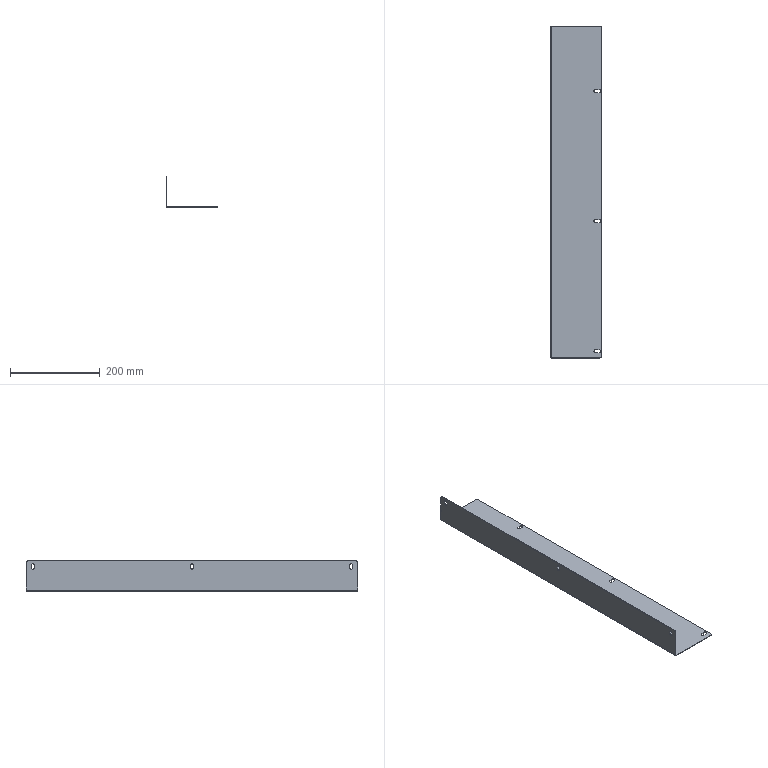Part | SolidWorks | features BaseBody 1 | 1 solid | 48 faces | box 115 x 740 x 67.2 mm | volume 159488 mm3 | cylinder 24 | plane 24 | commonest cylinder face diameters 7 x18 10 x4 2 x1 4.4 x1
STEP:
#1=CARTESIAN_POINT('',(55.,-355.,-1.2));
#2=VERTEX_POINT('',#1);
#3=CARTESIAN_POINT('',(51.5,-351.5,-1.2));
#4=VERTEX_POINT('',#3);
#5=CARTESIAN_POINT('',(51.5,-355.,-1.2));
#6=DIRECTION('',(0.,0.,1.));
#7=DIRECTION('',(1.,0.,0.));
#8=AXIS2_PLACEMENT_3D('',#5,#6,#7);
#9=CIRCLE('',#8,3.5);
#10=EDGE_CURVE('',#2,#4,#9,.T.);
#11=ORIENTED_EDGE('',*,*,#10,.F.);
#12=CARTESIAN_POINT('',(55.,-355.,0.));
#13=VERTEX_POINT('',#12);
#14=CARTESIAN_POINT('',(55.,-355.,-1.2));
#15=DIRECTION('',(0.,0.,1.));
#16=VECTOR('',#15,1000.);
#17=LINE('',#14,#16);
#18=EDGE_CURVE('',#2,#13,#17,.T.);
#19=ORIENTED_EDGE('',*,*,#18,.T.);
#20=CARTESIAN_POINT('',(51.5,-351.5,0.));
#21=VERTEX_POINT('',#20);
#22=CARTESIAN_POINT('',(51.5,-355.,0.));
#23=DIRECTION('',(0.,0.,1.));
#24=DIRECTION('',(1.,0.,0.));
#25=AXIS2_PLACEMENT_3D('',#22,#23,#24);
#26=CIRCLE('',#25,3.5);
#27=EDGE_CURVE('',#13,#21,#26,.T.);
#28=ORIENTED_EDGE('',*,*,#27,.T.);
#29=CARTESIAN_POINT('',(51.5,-351.5,-1.2));
#30=DIRECTION('',(0.,0.,1.));
#31=VECTOR('',#30,1000.);
#32=LINE('',#29,#31);
#33=EDGE_CURVE('',#4,#21,#32,.T.);
#34=ORIENTED_EDGE('',*,*,#33,.F.);
#35=EDGE_LOOP('',(#11,#19,#28,#34));
#36=FACE_OUTER_BOUND('',#35,.T.);
#37=CARTESIAN_POINT('',(51.5,-355.,-1.2));
#38=DIRECTION('',(0.,0.,1.));
#39=DIRECTION('',(1.,0.,0.));
#40=AXIS2_PLACEMENT_3D('',#37,#38,#39);
#41=CYLINDRICAL_SURFACE('',#40,3.5);
#42=ADVANCED_FACE('',(#36),#41,.F.);
#43=CARTESIAN_POINT('',(55.,-65.,-1.2));
#44=VERTEX_POINT('',#43);
#45=CARTESIAN_POINT('',(51.5,-61.5,-1.2));
#46=VERTEX_POINT('',#45);
#47=CARTESIAN_POINT('',(51.5,-65.,-1.2));
#48=DIRECTION('',(0.,0.,1.));
#49=DIRECTION('',(1.,0.,0.));
#50=AXIS2_PLACEMENT_3D('',#47,#48,#49);
#51=CIRCLE('',#50,3.5);
#52=EDGE_CURVE('',#44,#46,#51,.T.);
#53=ORIENTED_EDGE('',*,*,#52,.F.);
#54=CARTESIAN_POINT('',(55.,-65.,0.));
#55=VERTEX_POINT('',#54);
#56=CARTESIAN_POINT('',(55.,-65.,-1.2));
#57=DIRECTION('',(0.,0.,1.));
#58=VECTOR('',#57,1000.);
#59=LINE('',#56,#58);
#60=EDGE_CURVE('',#44,#55,#59,.T.);
#61=ORIENTED_EDGE('',*,*,#60,.T.);
#62=CARTESIAN_POINT('',(51.5,-61.5,0.));
#63=VERTEX_POINT('',#62);
#64=CARTESIAN_POINT('',(51.5,-65.,0.));
#65=DIRECTION('',(0.,0.,1.));
#66=DIRECTION('',(1.,0.,0.));
#67=AXIS2_PLACEMENT_3D('',#64,#65,#66);
#68=CIRCLE('',#67,3.5);
#69=EDGE_CURVE('',#55,#63,#68,.T.);
#70=ORIENTED_EDGE('',*,*,#69,.T.);
#71=CARTESIAN_POINT('',(51.5,-61.5,-1.2));
#72=DIRECTION('',(0.,0.,1.));
#73=VECTOR('',#72,1000.);
#74=LINE('',#71,#73);
#75=EDGE_CURVE('',#46,#63,#74,.T.);
#76=ORIENTED_EDGE('',*,*,#75,.F.);
#77=EDGE_LOOP('',(#53,#61,#70,#76));
#78=FACE_OUTER_BOUND('',#77,.T.);
#79=CARTESIAN_POINT('',(51.5,-65.,-1.2));
#80=DIRECTION('',(0.,0.,1.));
#81=DIRECTION('',(1.,0.,0.));
#82=AXIS2_PLACEMENT_3D('',#79,#80,#81);
#83=CYLINDRICAL_SURFACE('',#82,3.5);
#84=ADVANCED_FACE('',(#78),#83,.F.);
#85=CARTESIAN_POINT('',(55.,225.,-1.2));
#86=VERTEX_POINT('',#85);
#87=CARTESIAN_POINT('',(51.5,228.5,-1.2));
#88=VERTEX_POINT('',#87);
#89=CARTESIAN_POINT('',(51.5,225.,-1.2));
#90=DIRECTION('',(0.,0.,1.));
#91=DIRECTION('',(1.,0.,0.));
#92=AXIS2_PLACEMENT_3D('',#89,#90,#91);
#93=CIRCLE('',#92,3.5);
#94=EDGE_CURVE('',#86,#88,#93,.T.);
#95=ORIENTED_EDGE('',*,*,#94,.F.);
#96=CARTESIAN_POINT('',(55.,225.,0.));
#97=VERTEX_POINT('',#96);
#98=CARTESIAN_POINT('',(55.,225.,-1.2));
#99=DIRECTION('',(0.,0.,1.));
#100=VECTOR('',#99,1000.);
#101=LINE('',#98,#100);
#102=EDGE_CURVE('',#86,#97,#101,.T.);
#103=ORIENTED_EDGE('',*,*,#102,.T.);
#104=CARTESIAN_POINT('',(51.5,228.5,0.));
#105=VERTEX_POINT('',#104);
#106=CARTESIAN_POINT('',(51.5,225.,0.));
#107=DIRECTION('',(0.,0.,1.));
#108=DIRECTION('',(1.,0.,0.));
#109=AXIS2_PLACEMENT_3D('',#106,#107,#108);
#110=CIRCLE('',#109,3.5);
#111=EDGE_CURVE('',#97,#105,#110,.T.);
#112=ORIENTED_EDGE('',*,*,#111,.T.);
#113=CARTESIAN_POINT('',(51.5,228.5,-1.2));
#114=DIRECTION('',(0.,0.,1.));
#115=VECTOR('',#114,1000.);
#116=LINE('',#113,#115);
#117=EDGE_CURVE('',#88,#105,#116,.T.);
#118=ORIENTED_EDGE('',*,*,#117,.F.);
#119=EDGE_LOOP('',(#95,#103,#112,#118));
#120=FACE_OUTER_BOUND('',#119,.T.);
#121=CARTESIAN_POINT('',(51.5,225.,-1.2));
#122=DIRECTION('',(0.,0.,1.));
#123=DIRECTION('',(1.,0.,0.));
#124=AXIS2_PLACEMENT_3D('',#121,#122,#123);
#125=CYLINDRICAL_SURFACE('',#124,3.5);
#126=ADVANCED_FACE('',(#120),#125,.F.);
#127=CARTESIAN_POINT('',(-57.5,355.,47.5));
#128=VERTEX_POINT('',#127);
#129=CARTESIAN_POINT('',(-57.5,358.5,51.));
#130=VERTEX_POINT('',#129);
#131=CARTESIAN_POINT('',(-57.5,355.,51.));
#132=DIRECTION('',(1.,0.,0.));
#133=DIRECTION('',(0.,0.,-1.));
#134=AXIS2_PLACEMENT_3D('',#131,#132,#133);
#135=CIRCLE('',#134,3.5);
#136=EDGE_CURVE('',#128,#130,#135,.T.);
#137=ORIENTED_EDGE('',*,*,#136,.F.);
#138=CARTESIAN_POINT('',(-56.3,355.,47.5));
#139=VERTEX_POINT('',#138);
#140=CARTESIAN_POINT('',(-57.5,355.,47.5));
#141=DIRECTION('',(1.,0.,0.));
#142=VECTOR('',#141,1000.);
#143=LINE('',#140,#142);
#144=EDGE_CURVE('',#128,#139,#143,.T.);
#145=ORIENTED_EDGE('',*,*,#144,.T.);
#146=CARTESIAN_POINT('',(-56.3,358.5,51.));
#147=VERTEX_POINT('',#146);
#148=CARTESIAN_POINT('',(-56.3,355.,51.));
#149=DIRECTION('',(1.,0.,0.));
#150=DIRECTION('',(0.,0.,-1.));
#151=AXIS2_PLACEMENT_3D('',#148,#149,#150);
#152=CIRCLE('',#151,3.5);
#153=EDGE_CURVE('',#139,#147,#152,.T.);
#154=ORIENTED_EDGE('',*,*,#153,.T.);
#155=CARTESIAN_POINT('',(-57.5,358.5,51.));
#156=DIRECTION('',(1.,0.,0.));
#157=VECTOR('',#156,1000.);
#158=LINE('',#155,#157);
#159=EDGE_CURVE('',#130,#147,#158,.T.);
#160=ORIENTED_EDGE('',*,*,#159,.F.);
#161=EDGE_LOOP('',(#137,#145,#154,#160));
#162=FACE_OUTER_BOUND('',#161,.T.);
#163=CARTESIAN_POINT('',(-57.5,355.,51.));
#164=DIRECTION('',(1.,0.,0.));
#165=DIRECTION('',(0.,0.,-1.));
#166=AXIS2_PLACEMENT_3D('',#163,#164,#165);
#167=CYLINDRICAL_SURFACE('',#166,3.5);
#168=ADVANCED_FACE('',(#162),#167,.F.);
#169=CARTESIAN_POINT('',(-57.5,0.,47.5));
#170=VERTEX_POINT('',#169);
#171=CARTESIAN_POINT('',(-57.5,3.5,51.));
#172=VERTEX_POINT('',#171);
#173=CARTESIAN_POINT('',(-57.5,0.,51.));
#174=DIRECTION('',(1.,0.,0.));
#175=DIRECTION('',(0.,0.,-1.));
#176=AXIS2_PLACEMENT_3D('',#173,#174,#175);
#177=CIRCLE('',#176,3.5);
#178=EDGE_CURVE('',#170,#172,#177,.T.);
#179=ORIENTED_EDGE('',*,*,#178,.F.);
#180=CARTESIAN_POINT('',(-56.3,0.,47.5));
#181=VERTEX_POINT('',#180);
#182=CARTESIAN_POINT('',(-57.5,0.,47.5));
#183=DIRECTION('',(1.,0.,0.));
#184=VECTOR('',#183,1000.);
#185=LINE('',#182,#184);
#186=EDGE_CURVE('',#170,#181,#185,.T.);
#187=ORIENTED_EDGE('',*,*,#186,.T.);
#188=CARTESIAN_POINT('',(-56.3,3.5,51.));
#189=VERTEX_POINT('',#188);
#190=CARTESIAN_POINT('',(-56.3,0.,51.));
#191=DIRECTION('',(1.,0.,0.));
#192=DIRECTION('',(0.,0.,-1.));
#193=AXIS2_PLACEMENT_3D('',#190,#191,#192);
#194=CIRCLE('',#193,3.5);
#195=EDGE_CURVE('',#181,#189,#194,.T.);
#196=ORIENTED_EDGE('',*,*,#195,.T.);
#197=CARTESIAN_POINT('',(-57.5,3.5,51.));
#198=DIRECTION('',(1.,0.,0.));
#199=VECTOR('',#198,1000.);
#200=LINE('',#197,#199);
#201=EDGE_CURVE('',#172,#189,#200,.T.);
#202=ORIENTED_EDGE('',*,*,#201,.F.);
#203=EDGE_LOOP('',(#179,#187,#196,#202));
#204=FACE_OUTER_BOUND('',#203,.T.);
#205=CARTESIAN_POINT('',(-57.5,0.,51.));
#206=DIRECTION('',(1.,0.,0.));
#207=DIRECTION('',(0.,0.,-1.));
#208=AXIS2_PLACEMENT_3D('',#205,#206,#207);
#209=CYLINDRICAL_SURFACE('',#208,3.5);
#210=ADVANCED_FACE('',(#204),#209,.F.);
#211=CARTESIAN_POINT('',(-57.5,-355.,47.5));
#212=VERTEX_POINT('',#211);
#213=CARTESIAN_POINT('',(-57.5,-351.5,51.));
#214=VERTEX_POINT('',#213);
#215=CARTESIAN_POINT('',(-57.5,-355.,51.));
#216=DIRECTION('',(1.,0.,0.));
#217=DIRECTION('',(0.,0.,-1.));
#218=AXIS2_PLACEMENT_3D('',#215,#216,#217);
#219=CIRCLE('',#218,3.5);
#220=EDGE_CURVE('',#212,#214,#219,.T.);
#221=ORIENTED_EDGE('',*,*,#220,.F.);
#222=CARTESIAN_POINT('',(-56.3,-355.,47.5));
#223=VERTEX_POINT('',#222);
#224=CARTESIAN_POINT('',(-57.5,-355.,47.5));
#225=DIRECTION('',(1.,0.,0.));
#226=VECTOR('',#225,1000.);
#227=LINE('',#224,#226);
#228=EDGE_CURVE('',#212,#223,#227,.T.);
#229=ORIENTED_EDGE('',*,*,#228,.T.);
#230=CARTESIAN_POINT('',(-56.3,-351.5,51.));
#231=VERTEX_POINT('',#230);
#232=CARTESIAN_POINT('',(-56.3,-355.,51.));
#233=DIRECTION('',(1.,0.,0.));
#234=DIRECTION('',(0.,0.,-1.));
#235=AXIS2_PLACEMENT_3D('',#232,#233,#234);
#236=CIRCLE('',#235,3.5);
#237=EDGE_CURVE('',#223,#231,#236,.T.);
#238=ORIENTED_EDGE('',*,*,#237,.T.);
#239=CARTESIAN_POINT('',(-57.5,-351.5,51.));
#240=DIRECTION('',(1.,0.,0.));
#241=VECTOR('',#240,1000.);
#242=LINE('',#239,#241);
#243=EDGE_CURVE('',#214,#231,#242,.T.);
#244=ORIENTED_EDGE('',*,*,#243,.F.);
#245=EDGE_LOOP('',(#221,#229,#238,#244));
#246=FACE_OUTER_BOUND('',#245,.T.);
#247=CARTESIAN_POINT('',(-57.5,-355.,51.));
#248=DIRECTION('',(1.,0.,0.));
#249=DIRECTION('',(0.,0.,-1.));
#250=AXIS2_PLACEMENT_3D('',#247,#248,#249);
#251=CYLINDRICAL_SURFACE('',#250,3.5);
#252=ADVANCED_FACE('',(#246),#251,.F.);
#253=CARTESIAN_POINT('',(-55.3,-370.,-1.2));
#254=VERTEX_POINT('',#253);
#255=CARTESIAN_POINT('',(52.5,-370.,-1.2));
#256=VERTEX_POINT('',#255);
#257=CARTESIAN_POINT('',(-57.5,-370.,-1.2));
#258=DIRECTION('',(1.,0.,0.));
#259=VECTOR('',#258,1000.);
#260=LINE('',#257,#259);
#261=EDGE_CURVE('',#254,#256,#260,.T.);
#262=ORIENTED_EDGE('',*,*,#261,.T.);
#263=CARTESIAN_POINT('',(52.5,-370.,0.));
#264=VERTEX_POINT('',#263);
#265=CARTESIAN_POINT('',(52.5,-370.,-1.2));
#266=DIRECTION('',(0.,0.,1.));
#267=VECTOR('',#266,1000.);
#268=LINE('',#265,#267);
#269=EDGE_CURVE('',#256,#264,#268,.T.);
#270=ORIENTED_EDGE('',*,*,#269,.T.);
#271=CARTESIAN_POINT('',(-55.3,-370.,0.));
#272=VERTEX_POINT('',#271);
#273=CARTESIAN_POINT('',(-57.5,-370.,0.));
#274=DIRECTION('',(1.,0.,0.));
#275=VECTOR('',#274,1000.);
#276=LINE('',#273,#275);
#277=EDGE_CURVE('',#272,#264,#276,.T.);
#278=ORIENTED_EDGE('',*,*,#277,.F.);
#279=CARTESIAN_POINT('',(-55.3,-370.,0.));
#280=DIRECTION('',(0.,0.,-1.));
#281=VECTOR('',#280,1000.);
#282=LINE('',#279,#281);
#283=EDGE_CURVE('',#272,#254,#282,.T.);
#284=ORIENTED_EDGE('',*,*,#283,.T.);
#285=EDGE_LOOP('',(#262,#270,#278,#284));
#286=FACE_OUTER_BOUND('',#285,.T.);
#287=CARTESIAN_POINT('',(-57.5,-370.,-1.2));
#288=DIRECTION('',(0.,-1.,0.));
#289=DIRECTION('',(0.,0.,-1.));
#290=AXIS2_PLACEMENT_3D('',#287,#288,#289);
#291=PLANE('',#290);
#292=ADVANCED_FACE('',(#286),#291,.T.);
#293=CARTESIAN_POINT('',(43.5,-351.5,-1.2));
#294=VERTEX_POINT('',#293);
#295=CARTESIAN_POINT('',(43.5,-351.5,-1.2));
#296=DIRECTION('',(-1.,0.,0.));
#297=VECTOR('',#296,1000.);
#298=LINE('',#295,#297);
#299=EDGE_CURVE('',#4,#294,#298,.T.);
#300=ORIENTED_EDGE('',*,*,#299,.T.);
#301=CARTESIAN_POINT('',(43.5,-358.5,-1.2));
#302=VERTEX_POINT('',#301);
#303=CARTESIAN_POINT('',(43.5,-355.,-1.2));
#304=DIRECTION('',(0.,0.,1.));
#305=DIRECTION('',(1.,0.,0.));
#306=AXIS2_PLACEMENT_3D('',#303,#304,#305);
#307=CIRCLE('',#306,3.5);
#308=EDGE_CURVE('',#294,#302,#307,.T.);
#309=ORIENTED_EDGE('',*,*,#308,.T.);
#310=CARTESIAN_POINT('',(51.5,-358.5,-1.2));
#311=VERTEX_POINT('',#310);
#312=CARTESIAN_POINT('',(43.5,-358.5,-1.2));
#313=DIRECTION('',(1.,0.,0.));
#314=VECTOR('',#313,1000.);
#315=LINE('',#312,#314);
#316=EDGE_CURVE('',#302,#311,#315,.T.);
#317=ORIENTED_EDGE('',*,*,#316,.T.);
#318=CARTESIAN_POINT('',(51.5,-355.,-1.2));
#319=DIRECTION('',(0.,0.,1.));
#320=DIRECTION('',(1.,0.,0.));
#321=AXIS2_PLACEMENT_3D('',#318,#319,#320);
#322=CIRCLE('',#321,3.5);
#323=EDGE_CURVE('',#311,#2,#322,.T.);
#324=ORIENTED_EDGE('',*,*,#323,.T.);
#325=ORIENTED_EDGE('',*,*,#10,.T.);
#326=EDGE_LOOP('',(#300,#309,#317,#324,#325));
#327=FACE_BOUND('',#326,.T.);
#328=CARTESIAN_POINT('',(43.5,-61.5,-1.2));
#329=VERTEX_POINT('',#328);
#330=CARTESIAN_POINT('',(43.5,-61.5,-1.2));
#331=DIRECTION('',(-1.,0.,0.));
#332=VECTOR('',#331,1000.);
#333=LINE('',#330,#332);
#334=EDGE_CURVE('',#46,#329,#333,.T.);
#335=ORIENTED_EDGE('',*,*,#334,.T.);
#336=CARTESIAN_POINT('',(43.5,-68.5,-1.2));
#337=VERTEX_POINT('',#336);
#338=CARTESIAN_POINT('',(43.5,-65.,-1.2));
#339=DIRECTION('',(0.,0.,1.));
#340=DIRECTION('',(1.,0.,0.));
#341=AXIS2_PLACEMENT_3D('',#338,#339,#340);
#342=CIRCLE('',#341,3.5);
#343=EDGE_CURVE('',#329,#337,#342,.T.);
#344=ORIENTED_EDGE('',*,*,#343,.T.);
#345=CARTESIAN_POINT('',(51.5,-68.5,-1.2));
#346=VERTEX_POINT('',#345);
#347=CARTESIAN_POINT('',(43.5,-68.5,-1.2));
#348=DIRECTION('',(1.,0.,0.));
#349=VECTOR('',#348,1000.);
#350=LINE('',#347,#349);
#351=EDGE_CURVE('',#337,#346,#350,.T.);
#352=ORIENTED_EDGE('',*,*,#351,.T.);
#353=CARTESIAN_POINT('',(51.5,-65.,-1.2));
#354=DIRECTION('',(0.,0.,1.));
#355=DIRECTION('',(1.,0.,0.));
#356=AXIS2_PLACEMENT_3D('',#353,#354,#355);
#357=CIRCLE('',#356,3.5);
#358=EDGE_CURVE('',#346,#44,#357,.T.);
#359=ORIENTED_EDGE('',*,*,#358,.T.);
#360=ORIENTED_EDGE('',*,*,#52,.T.);
#361=EDGE_LOOP('',(#335,#344,#352,#359,#360));
#362=FACE_BOUND('',#361,.T.);
#363=CARTESIAN_POINT('',(43.5,228.5,-1.2));
#364=VERTEX_POINT('',#363);
#365=CARTESIAN_POINT('',(43.5,228.5,-1.2));
#366=DIRECTION('',(-1.,0.,0.));
#367=VECTOR('',#366,1000.);
#368=LINE('',#365,#367);
#369=EDGE_CURVE('',#88,#364,#368,.T.);
#370=ORIENTED_EDGE('',*,*,#369,.T.);
#371=CARTESIAN_POINT('',(43.5,221.5,-1.2));
#372=VERTEX_POINT('',#371);
#373=CARTESIAN_POINT('',(43.5,225.,-1.2));
#374=DIRECTION('',(0.,0.,1.));
#375=DIRECTION('',(1.,0.,0.));
#376=AXIS2_PLACEMENT_3D('',#373,#374,#375);
#377=CIRCLE('',#376,3.5);
#378=EDGE_CURVE('',#364,#372,#377,.T.);
#379=ORIENTED_EDGE('',*,*,#378,.T.);
#380=CARTESIAN_POINT('',(51.5,221.5,-1.2));
#381=VERTEX_POINT('',#380);
#382=CARTESIAN_POINT('',(43.5,221.5,-1.2));
#383=DIRECTION('',(1.,0.,0.));
#384=VECTOR('',#383,1000.);
#385=LINE('',#382,#384);
#386=EDGE_CURVE('',#372,#381,#385,.T.);
#387=ORIENTED_EDGE('',*,*,#386,.T.);
#388=CARTESIAN_POINT('',(51.5,225.,-1.2));
#389=DIRECTION('',(0.,0.,1.));
#390=DIRECTION('',(1.,0.,0.));
#391=AXIS2_PLACEMENT_3D('',#388,#389,#390);
#392=CIRCLE('',#391,3.5);
#393=EDGE_CURVE('',#381,#86,#392,.T.);
#394=ORIENTED_EDGE('',*,*,#393,.T.);
#395=ORIENTED_EDGE('',*,*,#94,.T.);
#396=EDGE_LOOP('',(#370,#379,#387,#394,#395));
#397=FACE_BOUND('',#396,.T.);
#398=CARTESIAN_POINT('',(57.5,-365.,-1.2));
#399=VERTEX_POINT('',#398);
#400=CARTESIAN_POINT('',(57.5,365.,-1.2));
#401=VERTEX_POINT('',#400);
#402=CARTESIAN_POINT('',(57.5,370.,-1.2));
#403=DIRECTION('',(0.,1.,0.));
#404=VECTOR('',#403,1000.);
#405=LINE('',#402,#404);
#406=EDGE_CURVE('',#399,#401,#405,.T.);
#407=ORIENTED_EDGE('',*,*,#406,.F.);
#408=CARTESIAN_POINT('',(52.5,-365.,-1.2));
#409=DIRECTION('',(0.,0.,-1.));
#410=DIRECTION('',(1.,0.,0.));
#411=AXIS2_PLACEMENT_3D('',#408,#409,#410);
#412=CIRCLE('',#411,5.);
#413=EDGE_CURVE('',#399,#256,#412,.T.);
#414=ORIENTED_EDGE('',*,*,#413,.T.);
#415=ORIENTED_EDGE('',*,*,#261,.F.);
#416=CARTESIAN_POINT('',(-55.3,370.,-1.2));
#417=VERTEX_POINT('',#416);
#418=CARTESIAN_POINT('',(-55.3,-370.,-1.2));
#419=DIRECTION('',(0.,1.,0.));
#420=VECTOR('',#419,1000.);
#421=LINE('',#418,#420);
#422=EDGE_CURVE('',#254,#417,#421,.T.);
#423=ORIENTED_EDGE('',*,*,#422,.T.);
#424=CARTESIAN_POINT('',(52.5,370.,-1.2));
#425=VERTEX_POINT('',#424);
#426=CARTESIAN_POINT('',(-57.5,370.,-1.2));
#427=DIRECTION('',(-1.,0.,0.));
#428=VECTOR('',#427,1000.);
#429=LINE('',#426,#428);
#430=EDGE_CURVE('',#425,#417,#429,.T.);
#431=ORIENTED_EDGE('',*,*,#430,.F.);
#432=CARTESIAN_POINT('',(52.5,365.,-1.2));
#433=DIRECTION('',(0.,0.,-1.));
#434=DIRECTION('',(1.,0.,0.));
#435=AXIS2_PLACEMENT_3D('',#432,#433,#434);
#436=CIRCLE('',#435,5.);
#437=EDGE_CURVE('',#425,#401,#436,.T.);
#438=ORIENTED_EDGE('',*,*,#437,.T.);
#439=EDGE_LOOP('',(#407,#414,#415,#423,#431,#438));
#440=FACE_OUTER_BOUND('',#439,.T.);
#441=CARTESIAN_POINT('',(0.,0.,-1.2));
#442=DIRECTION('',(0.,0.,1.));
#443=DIRECTION('',(1.,0.,0.));
#444=AXIS2_PLACEMENT_3D('',#441,#442,#443);
#445=PLANE('',#444);
#446=ADVANCED_FACE('',(#327,#362,#397,#440),#445,.F.);
#447=CARTESIAN_POINT('',(43.5,-351.5,0.));
#448=VERTEX_POINT('',#447);
#449=CARTESIAN_POINT('',(43.5,-358.5,0.));
#450=VERTEX_POINT('',#449);
#451=CARTESIAN_POINT('',(43.5,-355.,0.));
#452=DIRECTION('',(0.,0.,1.));
#453=DIRECTION('',(1.,0.,0.));
#454=AXIS2_PLACEMENT_3D('',#451,#452,#453);
#455=CIRCLE('',#454,3.5);
#456=EDGE_CURVE('',#448,#450,#455,.T.);
#457=ORIENTED_EDGE('',*,*,#456,.F.);
#458=CARTESIAN_POINT('',(43.5,-351.5,0.));
#459=DIRECTION('',(-1.,0.,0.));
#460=VECTOR('',#459,1000.);
#461=LINE('',#458,#460);
#462=EDGE_CURVE('',#21,#448,#461,.T.);
#463=ORIENTED_EDGE('',*,*,#462,.F.);
#464=ORIENTED_EDGE('',*,*,#27,.F.);
#465=CARTESIAN_POINT('',(51.5,-358.5,0.));
#466=VERTEX_POINT('',#465);
#467=CARTESIAN_POINT('',(51.5,-355.,0.));
#468=DIRECTION('',(0.,0.,1.));
#469=DIRECTION('',(1.,0.,0.));
#470=AXIS2_PLACEMENT_3D('',#467,#468,#469);
#471=CIRCLE('',#470,3.5);
#472=EDGE_CURVE('',#466,#13,#471,.T.);
#473=ORIENTED_EDGE('',*,*,#472,.F.);
#474=CARTESIAN_POINT('',(43.5,-358.5,0.));
#475=DIRECTION('',(1.,0.,0.));
#476=VECTOR('',#475,1000.);
#477=LINE('',#474,#476);
#478=EDGE_CURVE('',#450,#466,#477,.T.);
#479=ORIENTED_EDGE('',*,*,#478,.F.);
#480=EDGE_LOOP('',(#457,#463,#464,#473,#479));
#481=FACE_BOUND('',#480,.T.);
#482=CARTESIAN_POINT('',(43.5,-61.5,0.));
#483=VERTEX_POINT('',#482);
#484=CARTESIAN_POINT('',(43.5,-68.5,0.));
#485=VERTEX_POINT('',#484);
#486=CARTESIAN_POINT('',(43.5,-65.,0.));
#487=DIRECTION('',(0.,0.,1.));
#488=DIRECTION('',(1.,0.,0.));
#489=AXIS2_PLACEMENT_3D('',#486,#487,#488);
#490=CIRCLE('',#489,3.5);
#491=EDGE_CURVE('',#483,#485,#490,.T.);
#492=ORIENTED_EDGE('',*,*,#491,.F.);
#493=CARTESIAN_POINT('',(43.5,-61.5,0.));
#494=DIRECTION('',(-1.,0.,0.));
#495=VECTOR('',#494,1000.);
#496=LINE('',#493,#495);
#497=EDGE_CURVE('',#63,#483,#496,.T.);
#498=ORIENTED_EDGE('',*,*,#497,.F.);
#499=ORIENTED_EDGE('',*,*,#69,.F.);
#500=CARTESIAN_POINT('',(51.5,-68.5,0.));
#501=VERTEX_POINT('',#500);
#502=CARTESIAN_POINT('',(51.5,-65.,0.));
#503=DIRECTION('',(0.,0.,1.));
#504=DIRECTION('',(1.,0.,0.));
#505=AXIS2_PLACEMENT_3D('',#502,#503,#504);
#506=CIRCLE('',#505,3.5);
#507=EDGE_CURVE('',#501,#55,#506,.T.);
#508=ORIENTED_EDGE('',*,*,#507,.F.);
#509=CARTESIAN_POINT('',(43.5,-68.5,0.));
#510=DIRECTION('',(1.,0.,0.));
#511=VECTOR('',#510,1000.);
#512=LINE('',#509,#511);
#513=EDGE_CURVE('',#485,#501,#512,.T.);
#514=ORIENTED_EDGE('',*,*,#513,.F.);
#515=EDGE_LOOP('',(#492,#498,#499,#508,#514));
#516=FACE_BOUND('',#515,.T.);
#517=CARTESIAN_POINT('',(43.5,228.5,0.));
#518=VERTEX_POINT('',#517);
#519=CARTESIAN_POINT('',(43.5,221.5,0.));
#520=VERTEX_POINT('',#519);
#521=CARTESIAN_POINT('',(43.5,225.,0.));
#522=DIRECTION('',(0.,0.,1.));
#523=DIRECTION('',(1.,0.,0.));
#524=AXIS2_PLACEMENT_3D('',#521,#522,#523);
#525=CIRCLE('',#524,3.5);
#526=EDGE_CURVE('',#518,#520,#525,.T.);
#527=ORIENTED_EDGE('',*,*,#526,.F.);
#528=CARTESIAN_POINT('',(43.5,228.5,0.));
#529=DIRECTION('',(-1.,0.,0.));
#530=VECTOR('',#529,1000.);
#531=LINE('',#528,#530);
#532=EDGE_CURVE('',#105,#518,#531,.T.);
#533=ORIENTED_EDGE('',*,*,#532,.F.);
#534=ORIENTED_EDGE('',*,*,#111,.F.);
#535=CARTESIAN_POINT('',(51.5,221.5,0.));
#536=VERTEX_POINT('',#535);
#537=CARTESIAN_POINT('',(51.5,225.,0.));
#538=DIRECTION('',(0.,0.,1.));
#539=DIRECTION('',(1.,0.,0.));
#540=AXIS2_PLACEMENT_3D('',#537,#538,#539);
#541=CIRCLE('',#540,3.5);
#542=EDGE_CURVE('',#536,#97,#541,.T.);
#543=ORIENTED_EDGE('',*,*,#542,.F.);
#544=CARTESIAN_POINT('',(43.5,221.5,0.));
#545=DIRECTION('',(1.,0.,0.));
#546=VECTOR('',#545,1000.);
#547=LINE('',#544,#546);
#548=EDGE_CURVE('',#520,#536,#547,.T.);
#549=ORIENTED_EDGE('',*,*,#548,.F.);
#550=EDGE_LOOP('',(#527,#533,#534,#543,#549));
#551=FACE_BOUND('',#550,.T.);
#552=ORIENTED_EDGE('',*,*,#277,.T.);
#553=CARTESIAN_POINT('',(57.5,-365.,0.));
#554=VERTEX_POINT('',#553);
#555=CARTESIAN_POINT('',(52.5,-365.,0.));
#556=DIRECTION('',(0.,0.,1.));
#557=DIRECTION('',(1.,0.,0.));
#558=AXIS2_PLACEMENT_3D('',#555,#556,#557);
#559=CIRCLE('',#558,5.);
#560=EDGE_CURVE('',#264,#554,#559,.T.);
#561=ORIENTED_EDGE('',*,*,#560,.T.);
#562=CARTESIAN_POINT('',(57.5,365.,0.));
#563=VERTEX_POINT('',#562);
#564=CARTESIAN_POINT('',(57.5,370.,0.));
#565=DIRECTION('',(0.,1.,0.));
#566=VECTOR('',#565,1000.);
#567=LINE('',#564,#566);
#568=EDGE_CURVE('',#554,#563,#567,.T.);
#569=ORIENTED_EDGE('',*,*,#568,.T.);
#570=CARTESIAN_POINT('',(52.5,370.,0.));
#571=VERTEX_POINT('',#570);
#572=CARTESIAN_POINT('',(52.5,365.,0.));
#573=DIRECTION('',(0.,0.,1.));
#574=DIRECTION('',(1.,0.,0.));
#575=AXIS2_PLACEMENT_3D('',#572,#573,#574);
#576=CIRCLE('',#575,5.);
#577=EDGE_CURVE('',#563,#571,#576,.T.);
#578=ORIENTED_EDGE('',*,*,#577,.T.);
#579=CARTESIAN_POINT('',(-55.3,370.,0.));
#580=VERTEX_POINT('',#579);
#581=CARTESIAN_POINT('',(-57.5,370.,0.));
#582=DIRECTION('',(-1.,0.,0.));
#583=VECTOR('',#582,1000.);
#584=LINE('',#581,#583);
#585=EDGE_CURVE('',#571,#580,#584,.T.);
#586=ORIENTED_EDGE('',*,*,#585,.T.);
#587=CARTESIAN_POINT('',(-55.3,-370.,0.));
#588=DIRECTION('',(0.,1.,0.));
#589=VECTOR('',#588,1000.);
#590=LINE('',#587,#589);
#591=EDGE_CURVE('',#272,#580,#590,.T.);
#592=ORIENTED_EDGE('',*,*,#591,.F.);
#593=EDGE_LOOP('',(#552,#561,#569,#578,#586,#592));
#594=FACE_OUTER_BOUND('',#593,.T.);
#595=CARTESIAN_POINT('',(0.,0.,0.));
#596=DIRECTION('',(0.,0.,1.));
#597=DIRECTION('',(1.,0.,0.));
#598=AXIS2_PLACEMENT_3D('',#595,#596,#597);
#599=PLANE('',#598);
#600=ADVANCED_FACE('',(#481,#516,#551,#594),#599,.T.);
#601=ORIENTED_EDGE('',*,*,#568,.F.);
#602=CARTESIAN_POINT('',(57.5,-365.,-1.2));
#603=DIRECTION('',(0.,0.,-1.));
#604=VECTOR('',#603,1000.);
#605=LINE('',#602,#604);
#606=EDGE_CURVE('',#554,#399,#605,.T.);
#607=ORIENTED_EDGE('',*,*,#606,.T.);
#608=ORIENTED_EDGE('',*,*,#406,.T.);
#609=CARTESIAN_POINT('',(57.5,365.,-1.2));
#610=DIRECTION('',(0.,0.,1.));
#611=VECTOR('',#610,1000.);
#612=LINE('',#609,#611);
#613=EDGE_CURVE('',#401,#563,#612,.T.);
#614=ORIENTED_EDGE('',*,*,#613,.T.);
#615=EDGE_LOOP('',(#601,#607,#608,#614));
#616=FACE_OUTER_BOUND('',#615,.T.);
#617=CARTESIAN_POINT('',(57.5,370.,-1.2));
#618=DIRECTION('',(1.,0.,0.));
#619=DIRECTION('',(0.,1.,0.));
#620=AXIS2_PLACEMENT_3D('',#617,#618,#619);
#621=PLANE('',#620);
#622=ADVANCED_FACE('',(#616),#621,.T.);
#623=ORIENTED_EDGE('',*,*,#585,.F.);
#624=CARTESIAN_POINT('',(52.5,370.,-1.2));
#625=DIRECTION('',(0.,0.,-1.));
#626=VECTOR('',#625,1000.);
#627=LINE('',#624,#626);
#628=EDGE_CURVE('',#571,#425,#627,.T.);
#629=ORIENTED_EDGE('',*,*,#628,.T.);
#630=ORIENTED_EDGE('',*,*,#430,.T.);
#631=CARTESIAN_POINT('',(-55.3,370.,0.));
#632=DIRECTION('',(0.,0.,-1.));
#633=VECTOR('',#632,1000.);
#634=LINE('',#631,#633);
#635=EDGE_CURVE('',#580,#417,#634,.T.);
#636=ORIENTED_EDGE('',*,*,#635,.F.);
#637=EDGE_LOOP('',(#623,#629,#630,#636));
#638=FACE_OUTER_BOUND('',#637,.T.);
#639=CARTESIAN_POINT('',(-57.5,370.,-1.2));
#640=DIRECTION('',(0.,1.,0.));
#641=DIRECTION('',(0.,0.,1.));
#642=AXIS2_PLACEMENT_3D('',#639,#640,#641);
#643=PLANE('',#642);
#644=ADVANCED_FACE('',(#638),#643,.T.);
#645=CARTESIAN_POINT('',(-56.3,370.,1.));
#646=VERTEX_POINT('',#645);
#647=CARTESIAN_POINT('',(-57.5,370.,1.));
#648=VERTEX_POINT('',#647);
#649=CARTESIAN_POINT('',(-57.5,370.,1.));
#650=DIRECTION('',(-1.,0.,0.));
#651=VECTOR('',#650,1000.);
#652=LINE('',#649,#651);
#653=EDGE_CURVE('',#646,#648,#652,.T.);
#654=ORIENTED_EDGE('',*,*,#653,.F.);
#655=CARTESIAN_POINT('',(-55.3,370.,1.));
#656=DIRECTION('',(0.,1.,0.));
#657=DIRECTION('',(0.,0.,-1.));
#658=AXIS2_PLACEMENT_3D('',#655,#656,#657);
#659=CIRCLE('',#658,1.);
#660=EDGE_CURVE('',#580,#646,#659,.T.);
#661=ORIENTED_EDGE('',*,*,#660,.F.);
#662=ORIENTED_EDGE('',*,*,#635,.T.);
#663=CARTESIAN_POINT('',(-55.3,370.,1.));
#664=DIRECTION('',(0.,1.,0.));
#665=DIRECTION('',(0.,0.,-1.));
#666=AXIS2_PLACEMENT_3D('',#663,#664,#665);
#667=CIRCLE('',#666,2.2);
#668=EDGE_CURVE('',#417,#648,#667,.T.);
#669=ORIENTED_EDGE('',*,*,#668,.T.);
#670=EDGE_LOOP('',(#654,#661,#662,#669));
#671=FACE_OUTER_BOUND('',#670,.T.);
#672=CARTESIAN_POINT('',(-55.3,370.,1.));
#673=DIRECTION('',(0.,1.,0.));
#674=DIRECTION('',(0.,0.,1.));
#675=AXIS2_PLACEMENT_3D('',#672,#673,#674);
#676=PLANE('',#675);
#677=ADVANCED_FACE('',(#671),#676,.T.);
#678=CARTESIAN_POINT('',(-56.3,-370.,1.));
#679=VERTEX_POINT('',#678);
#680=CARTESIAN_POINT('',(-55.3,-370.,1.));
#681=DIRECTION('',(0.,-1.,0.));
#682=DIRECTION('',(0.,0.,-1.));
#683=AXIS2_PLACEMENT_3D('',#680,#681,#682);
#684=CIRCLE('',#683,1.);
#685=EDGE_CURVE('',#679,#272,#684,.T.);
#686=ORIENTED_EDGE('',*,*,#685,.F.);
#687=CARTESIAN_POINT('',(-57.5,-370.,1.));
#688=VERTEX_POINT('',#687);
#689=CARTESIAN_POINT('',(-56.3,-370.,1.));
#690=DIRECTION('',(-1.,0.,0.));
#691=VECTOR('',#690,1000.);
#692=LINE('',#689,#691);
#693=EDGE_CURVE('',#679,#688,#692,.T.);
#694=ORIENTED_EDGE('',*,*,#693,.T.);
#695=CARTESIAN_POINT('',(-55.3,-370.,1.));
#696=DIRECTION('',(0.,-1.,0.));
#697=DIRECTION('',(0.,0.,-1.));
#698=AXIS2_PLACEMENT_3D('',#695,#696,#697);
#699=CIRCLE('',#698,2.2);
#700=EDGE_CURVE('',#688,#254,#699,.T.);
#701=ORIENTED_EDGE('',*,*,#700,.T.);
#702=ORIENTED_EDGE('',*,*,#283,.F.);
#703=EDGE_LOOP('',(#686,#694,#701,#702));
#704=FACE_OUTER_BOUND('',#703,.T.);
#705=CARTESIAN_POINT('',(-55.3,-370.,1.));
#706=DIRECTION('',(0.,1.,0.));
#707=DIRECTION('',(0.,0.,1.));
#708=AXIS2_PLACEMENT_3D('',#705,#706,#707);
#709=PLANE('',#708);
#710=ADVANCED_FACE('',(#704),#709,.F.);
#711=ORIENTED_EDGE('',*,*,#422,.F.);
#712=ORIENTED_EDGE('',*,*,#700,.F.);
#713=CARTESIAN_POINT('',(-57.5,370.,1.));
#714=DIRECTION('',(0.,1.,0.));
#715=VECTOR('',#714,1000.);
#716=LINE('',#713,#715);
#717=EDGE_CURVE('',#688,#648,#716,.T.);
#718=ORIENTED_EDGE('',*,*,#717,.T.);
#719=ORIENTED_EDGE('',*,*,#668,.F.);
#720=EDGE_LOOP('',(#711,#712,#718,#719));
#721=FACE_OUTER_BOUND('',#720,.T.);
#722=CARTESIAN_POINT('',(-55.3,-370.,1.));
#723=DIRECTION('',(0.,-1.,0.));
#724=DIRECTION('',(-1.,0.,0.));
#725=AXIS2_PLACEMENT_3D('',#722,#723,#724);
#726=CYLINDRICAL_SURFACE('',#725,2.2);
#727=ADVANCED_FACE('',(#721),#726,.T.);
#728=ORIENTED_EDGE('',*,*,#591,.T.);
#729=ORIENTED_EDGE('',*,*,#660,.T.);
#730=CARTESIAN_POINT('',(-56.3,370.,1.));
#731=DIRECTION('',(0.,-1.,0.));
#732=VECTOR('',#731,1000.);
#733=LINE('',#730,#732);
#734=EDGE_CURVE('',#646,#679,#733,.T.);
#735=ORIENTED_EDGE('',*,*,#734,.T.);
#736=ORIENTED_EDGE('',*,*,#685,.T.);
#737=EDGE_LOOP('',(#728,#729,#735,#736));
#738=FACE_OUTER_BOUND('',#737,.T.);
#739=CARTESIAN_POINT('',(-55.3,-370.,1.));
#740=DIRECTION('',(0.,-1.,0.));
#741=DIRECTION('',(-1.,0.,0.));
#742=AXIS2_PLACEMENT_3D('',#739,#740,#741);
#743=CYLINDRICAL_SURFACE('',#742,1.);
#744=ADVANCED_FACE('',(#738),#743,.F.);
#745=CARTESIAN_POINT('',(-57.5,370.,61.));
#746=VERTEX_POINT('',#745);
#747=CARTESIAN_POINT('',(-57.5,370.,0.));
#748=DIRECTION('',(0.,0.,-1.));
#749=VECTOR('',#748,1000.);
#750=LINE('',#747,#749);
#751=EDGE_CURVE('',#746,#648,#750,.T.);
#752=ORIENTED_EDGE('',*,*,#751,.F.);
#753=CARTESIAN_POINT('',(-56.3,370.,61.));
#754=VERTEX_POINT('',#753);
#755=CARTESIAN_POINT('',(-57.5,370.,61.));
#756=DIRECTION('',(1.,0.,0.));
#757=VECTOR('',#756,1000.);
#758=LINE('',#755,#757);
#759=EDGE_CURVE('',#746,#754,#758,.T.);
#760=ORIENTED_EDGE('',*,*,#759,.T.);
#761=CARTESIAN_POINT('',(-56.3,370.,0.));
#762=DIRECTION('',(0.,0.,-1.));
#763=VECTOR('',#762,1000.);
#764=LINE('',#761,#763);
#765=EDGE_CURVE('',#754,#646,#764,.T.);
#766=ORIENTED_EDGE('',*,*,#765,.T.);
#767=ORIENTED_EDGE('',*,*,#653,.T.);
#768=EDGE_LOOP('',(#752,#760,#766,#767));
#769=FACE_OUTER_BOUND('',#768,.T.);
#770=CARTESIAN_POINT('',(-57.5,370.,0.));
#771=DIRECTION('',(0.,-1.,0.));
#772=DIRECTION('',(0.,0.,-1.));
#773=AXIS2_PLACEMENT_3D('',#770,#771,#772);
#774=PLANE('',#773);
#775=ADVANCED_FACE('',(#769),#774,.F.);
#776=CARTESIAN_POINT('',(-56.3,-370.,61.));
#777=VERTEX_POINT('',#776);
#778=CARTESIAN_POINT('',(-56.3,-370.,66.));
#779=DIRECTION('',(0.,0.,1.));
#780=VECTOR('',#779,1000.);
#781=LINE('',#778,#780);
#782=EDGE_CURVE('',#679,#777,#781,.T.);
#783=ORIENTED_EDGE('',*,*,#782,.T.);
#784=CARTESIAN_POINT('',(-57.5,-370.,61.));
#785=VERTEX_POINT('',#784);
#786=CARTESIAN_POINT('',(-57.5,-370.,61.));
#787=DIRECTION('',(-1.,0.,0.));
#788=VECTOR('',#787,1000.);
#789=LINE('',#786,#788);
#790=EDGE_CURVE('',#777,#785,#789,.T.);
#791=ORIENTED_EDGE('',*,*,#790,.T.);
#792=CARTESIAN_POINT('',(-57.5,-370.,0.));
#793=DIRECTION('',(0.,0.,1.));
#794=VECTOR('',#793,1000.);
#795=LINE('',#792,#794);
#796=EDGE_CURVE('',#688,#785,#795,.T.);
#797=ORIENTED_EDGE('',*,*,#796,.F.);
#798=ORIENTED_EDGE('',*,*,#693,.F.);
#799=EDGE_LOOP('',(#783,#791,#797,#798));
#800=FACE_OUTER_BOUND('',#799,.T.);
#801=CARTESIAN_POINT('',(-57.5,-370.,66.));
#802=DIRECTION('',(0.,1.,0.));
#803=DIRECTION('',(0.,0.,1.));
#804=AXIS2_PLACEMENT_3D('',#801,#802,#803);
#805=PLANE('',#804);
#806=ADVANCED_FACE('',(#800),#805,.F.);
#807=CARTESIAN_POINT('',(-57.5,358.5,56.));
#808=VERTEX_POINT('',#807);
#809=CARTESIAN_POINT('',(-57.5,358.5,56.));
#810=DIRECTION('',(0.,0.,1.));
#811=VECTOR('',#810,1000.);
#812=LINE('',#809,#811);
#813=EDGE_CURVE('',#130,#808,#812,.T.);
#814=ORIENTED_EDGE('',*,*,#813,.T.);
#815=CARTESIAN_POINT('',(-57.5,351.5,56.));
#816=VERTEX_POINT('',#815);
#817=CARTESIAN_POINT('',(-57.5,355.,56.));
#818=DIRECTION('',(1.,0.,0.));
#819=DIRECTION('',(0.,0.,-1.));
#820=AXIS2_PLACEMENT_3D('',#817,#818,#819);
#821=CIRCLE('',#820,3.5);
#822=EDGE_CURVE('',#808,#816,#821,.T.);
#823=ORIENTED_EDGE('',*,*,#822,.T.);
#824=CARTESIAN_POINT('',(-57.5,351.5,51.));
#825=VERTEX_POINT('',#824);
#826=CARTESIAN_POINT('',(-57.5,351.5,56.));
#827=DIRECTION('',(0.,0.,-1.));
#828=VECTOR('',#827,1000.);
#829=LINE('',#826,#828);
#830=EDGE_CURVE('',#816,#825,#829,.T.);
#831=ORIENTED_EDGE('',*,*,#830,.T.);
#832=CARTESIAN_POINT('',(-57.5,355.,51.));
#833=DIRECTION('',(1.,0.,0.));
#834=DIRECTION('',(0.,0.,-1.));
#835=AXIS2_PLACEMENT_3D('',#832,#833,#834);
#836=CIRCLE('',#835,3.5);
#837=EDGE_CURVE('',#825,#128,#836,.T.);
#838=ORIENTED_EDGE('',*,*,#837,.T.);
#839=ORIENTED_EDGE('',*,*,#136,.T.);
#840=EDGE_LOOP('',(#814,#823,#831,#838,#839));
#841=FACE_BOUND('',#840,.T.);
#842=CARTESIAN_POINT('',(-57.5,3.5,56.));
#843=VERTEX_POINT('',#842);
#844=CARTESIAN_POINT('',(-57.5,3.5,56.));
#845=DIRECTION('',(0.,0.,1.));
#846=VECTOR('',#845,1000.);
#847=LINE('',#844,#846);
#848=EDGE_CURVE('',#172,#843,#847,.T.);
#849=ORIENTED_EDGE('',*,*,#848,.T.);
#850=CARTESIAN_POINT('',(-57.5,-3.5,56.));
#851=VERTEX_POINT('',#850);
#852=CARTESIAN_POINT('',(-57.5,0.,56.));
#853=DIRECTION('',(1.,0.,0.));
#854=DIRECTION('',(0.,0.,-1.));
#855=AXIS2_PLACEMENT_3D('',#852,#853,#854);
#856=CIRCLE('',#855,3.5);
#857=EDGE_CURVE('',#843,#851,#856,.T.);
#858=ORIENTED_EDGE('',*,*,#857,.T.);
#859=CARTESIAN_POINT('',(-57.5,-3.5,51.));
#860=VERTEX_POINT('',#859);
#861=CARTESIAN_POINT('',(-57.5,-3.5,56.));
#862=DIRECTION('',(0.,0.,-1.));
#863=VECTOR('',#862,1000.);
#864=LINE('',#861,#863);
#865=EDGE_CURVE('',#851,#860,#864,.T.);
#866=ORIENTED_EDGE('',*,*,#865,.T.);
#867=CARTESIAN_POINT('',(-57.5,0.,51.));
#868=DIRECTION('',(1.,0.,0.));
#869=DIRECTION('',(0.,0.,-1.));
#870=AXIS2_PLACEMENT_3D('',#867,#868,#869);
#871=CIRCLE('',#870,3.5);
#872=EDGE_CURVE('',#860,#170,#871,.T.);
#873=ORIENTED_EDGE('',*,*,#872,.T.);
#874=ORIENTED_EDGE('',*,*,#178,.T.);
#875=EDGE_LOOP('',(#849,#858,#866,#873,#874));
#876=FACE_BOUND('',#875,.T.);
#877=CARTESIAN_POINT('',(-57.5,-351.5,56.));
#878=VERTEX_POINT('',#877);
#879=CARTESIAN_POINT('',(-57.5,-351.5,56.));
#880=DIRECTION('',(0.,0.,1.));
#881=VECTOR('',#880,1000.);
#882=LINE('',#879,#881);
#883=EDGE_CURVE('',#214,#878,#882,.T.);
#884=ORIENTED_EDGE('',*,*,#883,.T.);
#885=CARTESIAN_POINT('',(-57.5,-358.5,56.));
#886=VERTEX_POINT('',#885);
#887=CARTESIAN_POINT('',(-57.5,-355.,56.));
#888=DIRECTION('',(1.,0.,0.));
#889=DIRECTION('',(0.,0.,-1.));
#890=AXIS2_PLACEMENT_3D('',#887,#888,#889);
#891=CIRCLE('',#890,3.5);
#892=EDGE_CURVE('',#878,#886,#891,.T.);
#893=ORIENTED_EDGE('',*,*,#892,.T.);
#894=CARTESIAN_POINT('',(-57.5,-358.5,51.));
#895=VERTEX_POINT('',#894);
#896=CARTESIAN_POINT('',(-57.5,-358.5,56.));
#897=DIRECTION('',(0.,0.,-1.));
#898=VECTOR('',#897,1000.);
#899=LINE('',#896,#898);
#900=EDGE_CURVE('',#886,#895,#899,.T.);
#901=ORIENTED_EDGE('',*,*,#900,.T.);
#902=CARTESIAN_POINT('',(-57.5,-355.,51.));
#903=DIRECTION('',(1.,0.,0.));
#904=DIRECTION('',(0.,0.,-1.));
#905=AXIS2_PLACEMENT_3D('',#902,#903,#904);
#906=CIRCLE('',#905,3.5);
#907=EDGE_CURVE('',#895,#212,#906,.T.);
#908=ORIENTED_EDGE('',*,*,#907,.T.);
#909=ORIENTED_EDGE('',*,*,#220,.T.);
#910=EDGE_LOOP('',(#884,#893,#901,#908,#909));
#911=FACE_BOUND('',#910,.T.);
#912=ORIENTED_EDGE('',*,*,#796,.T.);
#913=CARTESIAN_POINT('',(-57.5,-365.,66.));
#914=VERTEX_POINT('',#913);
#915=CARTESIAN_POINT('',(-57.5,-365.,61.));
#916=DIRECTION('',(-1.,0.,0.));
#917=DIRECTION('',(0.,0.,-1.));
#918=AXIS2_PLACEMENT_3D('',#915,#916,#917);
#919=CIRCLE('',#918,5.);
#920=EDGE_CURVE('',#785,#914,#919,.T.);
#921=ORIENTED_EDGE('',*,*,#920,.T.);
#922=CARTESIAN_POINT('',(-57.5,365.,66.));
#923=VERTEX_POINT('',#922);
#924=CARTESIAN_POINT('',(-57.5,0.,66.));
#925=DIRECTION('',(0.,1.,0.));
#926=VECTOR('',#925,1000.);
#927=LINE('',#924,#926);
#928=EDGE_CURVE('',#914,#923,#927,.T.);
#929=ORIENTED_EDGE('',*,*,#928,.T.);
#930=CARTESIAN_POINT('',(-57.5,365.,61.));
#931=DIRECTION('',(-1.,0.,0.));
#932=DIRECTION('',(0.,0.,-1.));
#933=AXIS2_PLACEMENT_3D('',#930,#931,#932);
#934=CIRCLE('',#933,5.);
#935=EDGE_CURVE('',#923,#746,#934,.T.);
#936=ORIENTED_EDGE('',*,*,#935,.T.);
#937=ORIENTED_EDGE('',*,*,#751,.T.);
#938=ORIENTED_EDGE('',*,*,#717,.F.);
#939=EDGE_LOOP('',(#912,#921,#929,#936,#937,#938));
#940=FACE_OUTER_BOUND('',#939,.T.);
#941=CARTESIAN_POINT('',(-57.5,0.,0.));
#942=DIRECTION('',(1.,0.,0.));
#943=DIRECTION('',(0.,0.,-1.));
#944=AXIS2_PLACEMENT_3D('',#941,#942,#943);
#945=PLANE('',#944);
#946=ADVANCED_FACE('',(#841,#876,#911,#940),#945,.F.);
#947=CARTESIAN_POINT('',(-56.3,358.5,56.));
#948=VERTEX_POINT('',#947);
#949=CARTESIAN_POINT('',(-56.3,351.5,56.));
#950=VERTEX_POINT('',#949);
#951=CARTESIAN_POINT('',(-56.3,355.,56.));
#952=DIRECTION('',(1.,0.,0.));
#953=DIRECTION('',(0.,0.,-1.));
#954=AXIS2_PLACEMENT_3D('',#951,#952,#953);
#955=CIRCLE('',#954,3.5);
#956=EDGE_CURVE('',#948,#950,#955,.T.);
#957=ORIENTED_EDGE('',*,*,#956,.F.);
#958=CARTESIAN_POINT('',(-56.3,358.5,56.));
#959=DIRECTION('',(0.,0.,1.));
#960=VECTOR('',#959,1000.);
#961=LINE('',#958,#960);
#962=EDGE_CURVE('',#147,#948,#961,.T.);
#963=ORIENTED_EDGE('',*,*,#962,.F.);
#964=ORIENTED_EDGE('',*,*,#153,.F.);
#965=CARTESIAN_POINT('',(-56.3,351.5,51.));
#966=VERTEX_POINT('',#965);
#967=CARTESIAN_POINT('',(-56.3,355.,51.));
#968=DIRECTION('',(1.,0.,0.));
#969=DIRECTION('',(0.,0.,-1.));
#970=AXIS2_PLACEMENT_3D('',#967,#968,#969);
#971=CIRCLE('',#970,3.5);
#972=EDGE_CURVE('',#966,#139,#971,.T.);
#973=ORIENTED_EDGE('',*,*,#972,.F.);
#974=CARTESIAN_POINT('',(-56.3,351.5,56.));
#975=DIRECTION('',(0.,0.,-1.));
#976=VECTOR('',#975,1000.);
#977=LINE('',#974,#976);
#978=EDGE_CURVE('',#950,#966,#977,.T.);
#979=ORIENTED_EDGE('',*,*,#978,.F.);
#980=EDGE_LOOP('',(#957,#963,#964,#973,#979));
#981=FACE_BOUND('',#980,.T.);
#982=CARTESIAN_POINT('',(-56.3,3.5,56.));
#983=VERTEX_POINT('',#982);
#984=CARTESIAN_POINT('',(-56.3,-3.5,56.));
#985=VERTEX_POINT('',#984);
#986=CARTESIAN_POINT('',(-56.3,0.,56.));
#987=DIRECTION('',(1.,0.,0.));
#988=DIRECTION('',(0.,0.,-1.));
#989=AXIS2_PLACEMENT_3D('',#986,#987,#988);
#990=CIRCLE('',#989,3.5);
#991=EDGE_CURVE('',#983,#985,#990,.T.);
#992=ORIENTED_EDGE('',*,*,#991,.F.);
#993=CARTESIAN_POINT('',(-56.3,3.5,56.));
#994=DIRECTION('',(0.,0.,1.));
#995=VECTOR('',#994,1000.);
#996=LINE('',#993,#995);
#997=EDGE_CURVE('',#189,#983,#996,.T.);
#998=ORIENTED_EDGE('',*,*,#997,.F.);
#999=ORIENTED_EDGE('',*,*,#195,.F.);
#1000=CARTESIAN_POINT('',(-56.3,-3.5,51.));
#1001=VERTEX_POINT('',#1000);
#1002=CARTESIAN_POINT('',(-56.3,0.,51.));
#1003=DIRECTION('',(1.,0.,0.));
#1004=DIRECTION('',(0.,0.,-1.));
#1005=AXIS2_PLACEMENT_3D('',#1002,#1003,#1004);
#1006=CIRCLE('',#1005,3.5);
#1007=EDGE_CURVE('',#1001,#181,#1006,.T.);
#1008=ORIENTED_EDGE('',*,*,#1007,.F.);
#1009=CARTESIAN_POINT('',(-56.3,-3.5,56.));
#1010=DIRECTION('',(0.,0.,-1.));
#1011=VECTOR('',#1010,1000.);
#1012=LINE('',#1009,#1011);
#1013=EDGE_CURVE('',#985,#1001,#1012,.T.);
#1014=ORIENTED_EDGE('',*,*,#1013,.F.);
#1015=EDGE_LOOP('',(#992,#998,#999,#1008,#1014));
#1016=FACE_BOUND('',#1015,.T.);
#1017=CARTESIAN_POINT('',(-56.3,-351.5,56.));
#1018=VERTEX_POINT('',#1017);
#1019=CARTESIAN_POINT('',(-56.3,-358.5,56.));
#1020=VERTEX_POINT('',#1019);
#1021=CARTESIAN_POINT('',(-56.3,-355.,56.));
#1022=DIRECTION('',(1.,0.,0.));
#1023=DIRECTION('',(0.,0.,-1.));
#1024=AXIS2_PLACEMENT_3D('',#1021,#1022,#1023);
#1025=CIRCLE('',#1024,3.5);
#1026=EDGE_CURVE('',#1018,#1020,#1025,.T.);
#1027=ORIENTED_EDGE('',*,*,#1026,.F.);
#1028=CARTESIAN_POINT('',(-56.3,-351.5,56.));
#1029=DIRECTION('',(0.,0.,1.));
#1030=VECTOR('',#1029,1000.);
#1031=LINE('',#1028,#1030);
#1032=EDGE_CURVE('',#231,#1018,#1031,.T.);
#1033=ORIENTED_EDGE('',*,*,#1032,.F.);
#1034=ORIENTED_EDGE('',*,*,#237,.F.);
#1035=CARTESIAN_POINT('',(-56.3,-358.5,51.));
#1036=VERTEX_POINT('',#1035);
#1037=CARTESIAN_POINT('',(-56.3,-355.,51.));
#1038=DIRECTION('',(1.,0.,0.));
#1039=DIRECTION('',(0.,0.,-1.));
#1040=AXIS2_PLACEMENT_3D('',#1037,#1038,#1039);
#1041=CIRCLE('',#1040,3.5);
#1042=EDGE_CURVE('',#1036,#223,#1041,.T.);
#1043=ORIENTED_EDGE('',*,*,#1042,.F.);
#1044=CARTESIAN_POINT('',(-56.3,-358.5,56.));
#1045=DIRECTION('',(0.,0.,-1.));
#1046=VECTOR('',#1045,1000.);
#1047=LINE('',#1044,#1046);
#1048=EDGE_CURVE('',#1020,#1036,#1047,.T.);
#1049=ORIENTED_EDGE('',*,*,#1048,.F.);
#1050=EDGE_LOOP('',(#1027,#1033,#1034,#1043,#1049));
#1051=FACE_BOUND('',#1050,.T.);
#1052=CARTESIAN_POINT('',(-56.3,-365.,66.));
#1053=VERTEX_POINT('',#1052);
#1054=CARTESIAN_POINT('',(-56.3,365.,66.));
#1055=VERTEX_POINT('',#1054);
#1056=CARTESIAN_POINT('',(-56.3,370.,66.));
#1057=DIRECTION('',(0.,1.,0.));
#1058=VECTOR('',#1057,1000.);
#1059=LINE('',#1056,#1058);
#1060=EDGE_CURVE('',#1053,#1055,#1059,.T.);
#1061=ORIENTED_EDGE('',*,*,#1060,.F.);
#1062=CARTESIAN_POINT('',(-56.3,-365.,61.));
#1063=DIRECTION('',(1.,0.,0.));
#1064=DIRECTION('',(0.,0.,-1.));
#1065=AXIS2_PLACEMENT_3D('',#1062,#1063,#1064);
#1066=CIRCLE('',#1065,5.);
#1067=EDGE_CURVE('',#1053,#777,#1066,.T.);
#1068=ORIENTED_EDGE('',*,*,#1067,.T.);
#1069=ORIENTED_EDGE('',*,*,#782,.F.);
#1070=ORIENTED_EDGE('',*,*,#734,.F.);
#1071=ORIENTED_EDGE('',*,*,#765,.F.);
#1072=CARTESIAN_POINT('',(-56.3,365.,61.));
#1073=DIRECTION('',(1.,0.,0.));
#1074=DIRECTION('',(0.,0.,-1.));
#1075=AXIS2_PLACEMENT_3D('',#1072,#1073,#1074);
#1076=CIRCLE('',#1075,5.);
#1077=EDGE_CURVE('',#754,#1055,#1076,.T.);
#1078=ORIENTED_EDGE('',*,*,#1077,.T.);
#1079=EDGE_LOOP('',(#1061,#1068,#1069,#1070,#1071,#1078));
#1080=FACE_OUTER_BOUND('',#1079,.T.);
#1081=CARTESIAN_POINT('',(-56.3,0.,0.));
#1082=DIRECTION('',(1.,0.,0.));
#1083=DIRECTION('',(0.,0.,-1.));
#1084=AXIS2_PLACEMENT_3D('',#1081,#1082,#1083);
#1085=PLANE('',#1084);
#1086=ADVANCED_FACE('',(#981,#1016,#1051,#1080),#1085,.T.);
#1087=ORIENTED_EDGE('',*,*,#928,.F.);
#1088=CARTESIAN_POINT('',(-57.5,-365.,66.));
#1089=DIRECTION('',(1.,0.,0.));
#1090=VECTOR('',#1089,1000.);
#1091=LINE('',#1088,#1090);
#1092=EDGE_CURVE('',#914,#1053,#1091,.T.);
#1093=ORIENTED_EDGE('',*,*,#1092,.T.);
#1094=ORIENTED_EDGE('',*,*,#1060,.T.);
#1095=CARTESIAN_POINT('',(-57.5,365.,66.));
#1096=DIRECTION('',(-1.,0.,0.));
#1097=VECTOR('',#1096,1000.);
#1098=LINE('',#1095,#1097);
#1099=EDGE_CURVE('',#1055,#923,#1098,.T.);
#1100=ORIENTED_EDGE('',*,*,#1099,.T.);
#1101=EDGE_LOOP('',(#1087,#1093,#1094,#1100));
#1102=FACE_OUTER_BOUND('',#1101,.T.);
#1103=CARTESIAN_POINT('',(-57.5,370.,66.));
#1104=DIRECTION('',(0.,0.,-1.));
#1105=DIRECTION('',(-1.,0.,0.));
#1106=AXIS2_PLACEMENT_3D('',#1103,#1104,#1105);
#1107=PLANE('',#1106);
#1108=ADVANCED_FACE('',(#1102),#1107,.F.);
#1109=ORIENTED_EDGE('',*,*,#920,.F.);
#1110=ORIENTED_EDGE('',*,*,#790,.F.);
#1111=ORIENTED_EDGE('',*,*,#1067,.F.);
#1112=ORIENTED_EDGE('',*,*,#1092,.F.);
#1113=EDGE_LOOP('',(#1109,#1110,#1111,#1112));
#1114=FACE_OUTER_BOUND('',#1113,.T.);
#1115=CARTESIAN_POINT('',(-57.5,-365.,61.));
#1116=DIRECTION('',(1.,0.,0.));
#1117=DIRECTION('',(0.,0.,-1.));
#1118=AXIS2_PLACEMENT_3D('',#1115,#1116,#1117);
#1119=CYLINDRICAL_SURFACE('',#1118,5.);
#1120=ADVANCED_FACE('',(#1114),#1119,.T.);
#1121=ORIENTED_EDGE('',*,*,#413,.F.);
#1122=ORIENTED_EDGE('',*,*,#606,.F.);
#1123=ORIENTED_EDGE('',*,*,#560,.F.);
#1124=ORIENTED_EDGE('',*,*,#269,.F.);
#1125=EDGE_LOOP('',(#1121,#1122,#1123,#1124));
#1126=FACE_OUTER_BOUND('',#1125,.T.);
#1127=CARTESIAN_POINT('',(52.5,-365.,-1.2));
#1128=DIRECTION('',(0.,0.,1.));
#1129=DIRECTION('',(1.,0.,0.));
#1130=AXIS2_PLACEMENT_3D('',#1127,#1128,#1129);
#1131=CYLINDRICAL_SURFACE('',#1130,5.);
#1132=ADVANCED_FACE('',(#1126),#1131,.T.);
#1133=ORIENTED_EDGE('',*,*,#437,.F.);
#1134=ORIENTED_EDGE('',*,*,#628,.F.);
#1135=ORIENTED_EDGE('',*,*,#577,.F.);
#1136=ORIENTED_EDGE('',*,*,#613,.F.);
#1137=EDGE_LOOP('',(#1133,#1134,#1135,#1136));
#1138=FACE_OUTER_BOUND('',#1137,.T.);
#1139=CARTESIAN_POINT('',(52.5,365.,-1.2));
#1140=DIRECTION('',(0.,0.,1.));
#1141=DIRECTION('',(1.,0.,0.));
#1142=AXIS2_PLACEMENT_3D('',#1139,#1140,#1141);
#1143=CYLINDRICAL_SURFACE('',#1142,5.);
#1144=ADVANCED_FACE('',(#1138),#1143,.T.);
#1145=ORIENTED_EDGE('',*,*,#935,.F.);
#1146=ORIENTED_EDGE('',*,*,#1099,.F.);
#1147=ORIENTED_EDGE('',*,*,#1077,.F.);
#1148=ORIENTED_EDGE('',*,*,#759,.F.);
#1149=EDGE_LOOP('',(#1145,#1146,#1147,#1148));
#1150=FACE_OUTER_BOUND('',#1149,.T.);
#1151=CARTESIAN_POINT('',(-57.5,365.,61.));
#1152=DIRECTION('',(1.,0.,0.));
#1153=DIRECTION('',(0.,0.,-1.));
#1154=AXIS2_PLACEMENT_3D('',#1151,#1152,#1153);
#1155=CYLINDRICAL_SURFACE('',#1154,5.);
#1156=ADVANCED_FACE('',(#1150),#1155,.T.);
#1157=ORIENTED_EDGE('',*,*,#1026,.T.);
#1158=CARTESIAN_POINT('',(-57.5,-358.5,56.));
#1159=DIRECTION('',(1.,0.,0.));
#1160=VECTOR('',#1159,1000.);
#1161=LINE('',#1158,#1160);
#1162=EDGE_CURVE('',#886,#1020,#1161,.T.);
#1163=ORIENTED_EDGE('',*,*,#1162,.F.);
#1164=ORIENTED_EDGE('',*,*,#892,.F.);
#1165=CARTESIAN_POINT('',(-57.5,-351.5,56.));
#1166=DIRECTION('',(1.,0.,0.));
#1167=VECTOR('',#1166,1000.);
#1168=LINE('',#1165,#1167);
#1169=EDGE_CURVE('',#878,#1018,#1168,.T.);
#1170=ORIENTED_EDGE('',*,*,#1169,.T.);
#1171=EDGE_LOOP('',(#1157,#1163,#1164,#1170));
#1172=FACE_OUTER_BOUND('',#1171,.T.);
#1173=CARTESIAN_POINT('',(-57.5,-355.,56.));
#1174=DIRECTION('',(1.,0.,0.));
#1175=DIRECTION('',(0.,0.,-1.));
#1176=AXIS2_PLACEMENT_3D('',#1173,#1174,#1175);
#1177=CYLINDRICAL_SURFACE('',#1176,3.5);
#1178=ADVANCED_FACE('',(#1172),#1177,.F.);
#1179=ORIENTED_EDGE('',*,*,#1032,.T.);
#1180=ORIENTED_EDGE('',*,*,#1169,.F.);
#1181=ORIENTED_EDGE('',*,*,#883,.F.);
#1182=ORIENTED_EDGE('',*,*,#243,.T.);
#1183=EDGE_LOOP('',(#1179,#1180,#1181,#1182));
#1184=FACE_OUTER_BOUND('',#1183,.T.);
#1185=CARTESIAN_POINT('',(-57.5,-351.5,56.));
#1186=DIRECTION('',(0.,1.,0.));
#1187=DIRECTION('',(-1.,0.,0.));
#1188=AXIS2_PLACEMENT_3D('',#1185,#1186,#1187);
#1189=PLANE('',#1188);
#1190=ADVANCED_FACE('',(#1184),#1189,.F.);
#1191=ORIENTED_EDGE('',*,*,#228,.F.);
#1192=ORIENTED_EDGE('',*,*,#907,.F.);
#1193=CARTESIAN_POINT('',(-57.5,-358.5,51.));
#1194=DIRECTION('',(1.,0.,0.));
#1195=VECTOR('',#1194,1000.);
#1196=LINE('',#1193,#1195);
#1197=EDGE_CURVE('',#895,#1036,#1196,.T.);
#1198=ORIENTED_EDGE('',*,*,#1197,.T.);
#1199=ORIENTED_EDGE('',*,*,#1042,.T.);
#1200=EDGE_LOOP('',(#1191,#1192,#1198,#1199));
#1201=FACE_OUTER_BOUND('',#1200,.T.);
#1202=CARTESIAN_POINT('',(-57.5,-355.,51.));
#1203=DIRECTION('',(1.,0.,0.));
#1204=DIRECTION('',(0.,0.,-1.));
#1205=AXIS2_PLACEMENT_3D('',#1202,#1203,#1204);
#1206=CYLINDRICAL_SURFACE('',#1205,3.5);
#1207=ADVANCED_FACE('',(#1201),#1206,.F.);
#1208=ORIENTED_EDGE('',*,*,#1048,.T.);
#1209=ORIENTED_EDGE('',*,*,#1197,.F.);
#1210=ORIENTED_EDGE('',*,*,#900,.F.);
#1211=ORIENTED_EDGE('',*,*,#1162,.T.);
#1212=EDGE_LOOP('',(#1208,#1209,#1210,#1211));
#1213=FACE_OUTER_BOUND('',#1212,.T.);
#1214=CARTESIAN_POINT('',(-57.5,-358.5,56.));
#1215=DIRECTION('',(0.,-1.,0.));
#1216=DIRECTION('',(1.,0.,0.));
#1217=AXIS2_PLACEMENT_3D('',#1214,#1215,#1216);
#1218=PLANE('',#1217);
#1219=ADVANCED_FACE('',(#1213),#1218,.F.);
#1220=ORIENTED_EDGE('',*,*,#991,.T.);
#1221=CARTESIAN_POINT('',(-57.5,-3.5,56.));
#1222=DIRECTION('',(1.,0.,0.));
#1223=VECTOR('',#1222,1000.);
#1224=LINE('',#1221,#1223);
#1225=EDGE_CURVE('',#851,#985,#1224,.T.);
#1226=ORIENTED_EDGE('',*,*,#1225,.F.);
#1227=ORIENTED_EDGE('',*,*,#857,.F.);
#1228=CARTESIAN_POINT('',(-57.5,3.5,56.));
#1229=DIRECTION('',(1.,0.,0.));
#1230=VECTOR('',#1229,1000.);
#1231=LINE('',#1228,#1230);
#1232=EDGE_CURVE('',#843,#983,#1231,.T.);
#1233=ORIENTED_EDGE('',*,*,#1232,.T.);
#1234=EDGE_LOOP('',(#1220,#1226,#1227,#1233));
#1235=FACE_OUTER_BOUND('',#1234,.T.);
#1236=CARTESIAN_POINT('',(-57.5,0.,56.));
#1237=DIRECTION('',(1.,0.,0.));
#1238=DIRECTION('',(0.,0.,-1.));
#1239=AXIS2_PLACEMENT_3D('',#1236,#1237,#1238);
#1240=CYLINDRICAL_SURFACE('',#1239,3.5);
#1241=ADVANCED_FACE('',(#1235),#1240,.F.);
#1242=ORIENTED_EDGE('',*,*,#997,.T.);
#1243=ORIENTED_EDGE('',*,*,#1232,.F.);
#1244=ORIENTED_EDGE('',*,*,#848,.F.);
#1245=ORIENTED_EDGE('',*,*,#201,.T.);
#1246=EDGE_LOOP('',(#1242,#1243,#1244,#1245));
#1247=FACE_OUTER_BOUND('',#1246,.T.);
#1248=CARTESIAN_POINT('',(-57.5,3.5,56.));
#1249=DIRECTION('',(0.,1.,0.));
#1250=DIRECTION('',(-1.,0.,0.));
#1251=AXIS2_PLACEMENT_3D('',#1248,#1249,#1250);
#1252=PLANE('',#1251);
#1253=ADVANCED_FACE('',(#1247),#1252,.F.);
#1254=ORIENTED_EDGE('',*,*,#186,.F.);
#1255=ORIENTED_EDGE('',*,*,#872,.F.);
#1256=CARTESIAN_POINT('',(-57.5,-3.5,51.));
#1257=DIRECTION('',(1.,0.,0.));
#1258=VECTOR('',#1257,1000.);
#1259=LINE('',#1256,#1258);
#1260=EDGE_CURVE('',#860,#1001,#1259,.T.);
#1261=ORIENTED_EDGE('',*,*,#1260,.T.);
#1262=ORIENTED_EDGE('',*,*,#1007,.T.);
#1263=EDGE_LOOP('',(#1254,#1255,#1261,#1262));
#1264=FACE_OUTER_BOUND('',#1263,.T.);
#1265=CARTESIAN_POINT('',(-57.5,0.,51.));
#1266=DIRECTION('',(1.,0.,0.));
#1267=DIRECTION('',(0.,0.,-1.));
#1268=AXIS2_PLACEMENT_3D('',#1265,#1266,#1267);
#1269=CYLINDRICAL_SURFACE('',#1268,3.5);
#1270=ADVANCED_FACE('',(#1264),#1269,.F.);
#1271=ORIENTED_EDGE('',*,*,#1013,.T.);
#1272=ORIENTED_EDGE('',*,*,#1260,.F.);
#1273=ORIENTED_EDGE('',*,*,#865,.F.);
#1274=ORIENTED_EDGE('',*,*,#1225,.T.);
#1275=EDGE_LOOP('',(#1271,#1272,#1273,#1274));
#1276=FACE_OUTER_BOUND('',#1275,.T.);
#1277=CARTESIAN_POINT('',(-57.5,-3.5,56.));
#1278=DIRECTION('',(0.,-1.,0.));
#1279=DIRECTION('',(1.,0.,0.));
#1280=AXIS2_PLACEMENT_3D('',#1277,#1278,#1279);
#1281=PLANE('',#1280);
#1282=ADVANCED_FACE('',(#1276),#1281,.F.);
#1283=ORIENTED_EDGE('',*,*,#956,.T.);
#1284=CARTESIAN_POINT('',(-57.5,351.5,56.));
#1285=DIRECTION('',(1.,0.,0.));
#1286=VECTOR('',#1285,1000.);
#1287=LINE('',#1284,#1286);
#1288=EDGE_CURVE('',#816,#950,#1287,.T.);
#1289=ORIENTED_EDGE('',*,*,#1288,.F.);
#1290=ORIENTED_EDGE('',*,*,#822,.F.);
#1291=CARTESIAN_POINT('',(-57.5,358.5,56.));
#1292=DIRECTION('',(1.,0.,0.));
#1293=VECTOR('',#1292,1000.);
#1294=LINE('',#1291,#1293);
#1295=EDGE_CURVE('',#808,#948,#1294,.T.);
#1296=ORIENTED_EDGE('',*,*,#1295,.T.);
#1297=EDGE_LOOP('',(#1283,#1289,#1290,#1296));
#1298=FACE_OUTER_BOUND('',#1297,.T.);
#1299=CARTESIAN_POINT('',(-57.5,355.,56.));
#1300=DIRECTION('',(1.,0.,0.));
#1301=DIRECTION('',(0.,0.,-1.));
#1302=AXIS2_PLACEMENT_3D('',#1299,#1300,#1301);
#1303=CYLINDRICAL_SURFACE('',#1302,3.5);
#1304=ADVANCED_FACE('',(#1298),#1303,.F.);
#1305=ORIENTED_EDGE('',*,*,#962,.T.);
#1306=ORIENTED_EDGE('',*,*,#1295,.F.);
#1307=ORIENTED_EDGE('',*,*,#813,.F.);
#1308=ORIENTED_EDGE('',*,*,#159,.T.);
#1309=EDGE_LOOP('',(#1305,#1306,#1307,#1308));
#1310=FACE_OUTER_BOUND('',#1309,.T.);
#1311=CARTESIAN_POINT('',(-57.5,358.5,56.));
#1312=DIRECTION('',(0.,1.,0.));
#1313=DIRECTION('',(-1.,0.,0.));
#1314=AXIS2_PLACEMENT_3D('',#1311,#1312,#1313);
#1315=PLANE('',#1314);
#1316=ADVANCED_FACE('',(#1310),#1315,.F.);
#1317=ORIENTED_EDGE('',*,*,#144,.F.);
#1318=ORIENTED_EDGE('',*,*,#837,.F.);
#1319=CARTESIAN_POINT('',(-57.5,351.5,51.));
#1320=DIRECTION('',(1.,0.,0.));
#1321=VECTOR('',#1320,1000.);
#1322=LINE('',#1319,#1321);
#1323=EDGE_CURVE('',#825,#966,#1322,.T.);
#1324=ORIENTED_EDGE('',*,*,#1323,.T.);
#1325=ORIENTED_EDGE('',*,*,#972,.T.);
#1326=EDGE_LOOP('',(#1317,#1318,#1324,#1325));
#1327=FACE_OUTER_BOUND('',#1326,.T.);
#1328=CARTESIAN_POINT('',(-57.5,355.,51.));
#1329=DIRECTION('',(1.,0.,0.));
#1330=DIRECTION('',(0.,0.,-1.));
#1331=AXIS2_PLACEMENT_3D('',#1328,#1329,#1330);
#1332=CYLINDRICAL_SURFACE('',#1331,3.5);
#1333=ADVANCED_FACE('',(#1327),#1332,.F.);
#1334=ORIENTED_EDGE('',*,*,#978,.T.);
#1335=ORIENTED_EDGE('',*,*,#1323,.F.);
#1336=ORIENTED_EDGE('',*,*,#830,.F.);
#1337=ORIENTED_EDGE('',*,*,#1288,.T.);
#1338=EDGE_LOOP('',(#1334,#1335,#1336,#1337));
#1339=FACE_OUTER_BOUND('',#1338,.T.);
#1340=CARTESIAN_POINT('',(-57.5,351.5,56.));
#1341=DIRECTION('',(0.,-1.,0.));
#1342=DIRECTION('',(1.,0.,0.));
#1343=AXIS2_PLACEMENT_3D('',#1340,#1341,#1342);
#1344=PLANE('',#1343);
#1345=ADVANCED_FACE('',(#1339),#1344,.F.);
#1346=ORIENTED_EDGE('',*,*,#526,.T.);
#1347=CARTESIAN_POINT('',(43.5,221.5,-1.2));
#1348=DIRECTION('',(0.,0.,1.));
#1349=VECTOR('',#1348,1000.);
#1350=LINE('',#1347,#1349);
#1351=EDGE_CURVE('',#372,#520,#1350,.T.);
#1352=ORIENTED_EDGE('',*,*,#1351,.F.);
#1353=ORIENTED_EDGE('',*,*,#378,.F.);
#1354=CARTESIAN_POINT('',(43.5,228.5,-1.2));
#1355=DIRECTION('',(0.,0.,1.));
#1356=VECTOR('',#1355,1000.);
#1357=LINE('',#1354,#1356);
#1358=EDGE_CURVE('',#364,#518,#1357,.T.);
#1359=ORIENTED_EDGE('',*,*,#1358,.T.);
#1360=EDGE_LOOP('',(#1346,#1352,#1353,#1359));
#1361=FACE_OUTER_BOUND('',#1360,.T.);
#1362=CARTESIAN_POINT('',(43.5,225.,-1.2));
#1363=DIRECTION('',(0.,0.,1.));
#1364=DIRECTION('',(1.,0.,0.));
#1365=AXIS2_PLACEMENT_3D('',#1362,#1363,#1364);
#1366=CYLINDRICAL_SURFACE('',#1365,3.5);
#1367=ADVANCED_FACE('',(#1361),#1366,.F.);
#1368=ORIENTED_EDGE('',*,*,#532,.T.);
#1369=ORIENTED_EDGE('',*,*,#1358,.F.);
#1370=ORIENTED_EDGE('',*,*,#369,.F.);
#1371=ORIENTED_EDGE('',*,*,#117,.T.);
#1372=EDGE_LOOP('',(#1368,#1369,#1370,#1371));
#1373=FACE_OUTER_BOUND('',#1372,.T.);
#1374=CARTESIAN_POINT('',(43.5,228.5,-1.2));
#1375=DIRECTION('',(0.,1.,0.));
#1376=DIRECTION('',(0.,0.,1.));
#1377=AXIS2_PLACEMENT_3D('',#1374,#1375,#1376);
#1378=PLANE('',#1377);
#1379=ADVANCED_FACE('',(#1373),#1378,.F.);
#1380=ORIENTED_EDGE('',*,*,#102,.F.);
#1381=ORIENTED_EDGE('',*,*,#393,.F.);
#1382=CARTESIAN_POINT('',(51.5,221.5,-1.2));
#1383=DIRECTION('',(0.,0.,1.));
#1384=VECTOR('',#1383,1000.);
#1385=LINE('',#1382,#1384);
#1386=EDGE_CURVE('',#381,#536,#1385,.T.);
#1387=ORIENTED_EDGE('',*,*,#1386,.T.);
#1388=ORIENTED_EDGE('',*,*,#542,.T.);
#1389=EDGE_LOOP('',(#1380,#1381,#1387,#1388));
#1390=FACE_OUTER_BOUND('',#1389,.T.);
#1391=CARTESIAN_POINT('',(51.5,225.,-1.2));
#1392=DIRECTION('',(0.,0.,1.));
#1393=DIRECTION('',(1.,0.,0.));
#1394=AXIS2_PLACEMENT_3D('',#1391,#1392,#1393);
#1395=CYLINDRICAL_SURFACE('',#1394,3.5);
#1396=ADVANCED_FACE('',(#1390),#1395,.F.);
#1397=ORIENTED_EDGE('',*,*,#548,.T.);
#1398=ORIENTED_EDGE('',*,*,#1386,.F.);
#1399=ORIENTED_EDGE('',*,*,#386,.F.);
#1400=ORIENTED_EDGE('',*,*,#1351,.T.);
#1401=EDGE_LOOP('',(#1397,#1398,#1399,#1400));
#1402=FACE_OUTER_BOUND('',#1401,.T.);
#1403=CARTESIAN_POINT('',(43.5,221.5,-1.2));
#1404=DIRECTION('',(0.,-1.,0.));
#1405=DIRECTION('',(0.,0.,-1.));
#1406=AXIS2_PLACEMENT_3D('',#1403,#1404,#1405);
#1407=PLANE('',#1406);
#1408=ADVANCED_FACE('',(#1402),#1407,.F.);
#1409=ORIENTED_EDGE('',*,*,#491,.T.);
#1410=CARTESIAN_POINT('',(43.5,-68.5,-1.2));
#1411=DIRECTION('',(0.,0.,1.));
#1412=VECTOR('',#1411,1000.);
#1413=LINE('',#1410,#1412);
#1414=EDGE_CURVE('',#337,#485,#1413,.T.);
#1415=ORIENTED_EDGE('',*,*,#1414,.F.);
#1416=ORIENTED_EDGE('',*,*,#343,.F.);
#1417=CARTESIAN_POINT('',(43.5,-61.5,-1.2));
#1418=DIRECTION('',(0.,0.,1.));
#1419=VECTOR('',#1418,1000.);
#1420=LINE('',#1417,#1419);
#1421=EDGE_CURVE('',#329,#483,#1420,.T.);
#1422=ORIENTED_EDGE('',*,*,#1421,.T.);
#1423=EDGE_LOOP('',(#1409,#1415,#1416,#1422));
#1424=FACE_OUTER_BOUND('',#1423,.T.);
#1425=CARTESIAN_POINT('',(43.5,-65.,-1.2));
#1426=DIRECTION('',(0.,0.,1.));
#1427=DIRECTION('',(1.,0.,0.));
#1428=AXIS2_PLACEMENT_3D('',#1425,#1426,#1427);
#1429=CYLINDRICAL_SURFACE('',#1428,3.5);
#1430=ADVANCED_FACE('',(#1424),#1429,.F.);
#1431=ORIENTED_EDGE('',*,*,#497,.T.);
#1432=ORIENTED_EDGE('',*,*,#1421,.F.);
#1433=ORIENTED_EDGE('',*,*,#334,.F.);
#1434=ORIENTED_EDGE('',*,*,#75,.T.);
#1435=EDGE_LOOP('',(#1431,#1432,#1433,#1434));
#1436=FACE_OUTER_BOUND('',#1435,.T.);
#1437=CARTESIAN_POINT('',(43.5,-61.5,-1.2));
#1438=DIRECTION('',(0.,1.,0.));
#1439=DIRECTION('',(0.,0.,1.));
#1440=AXIS2_PLACEMENT_3D('',#1437,#1438,#1439);
#1441=PLANE('',#1440);
#1442=ADVANCED_FACE('',(#1436),#1441,.F.);
#1443=ORIENTED_EDGE('',*,*,#60,.F.);
#1444=ORIENTED_EDGE('',*,*,#358,.F.);
#1445=CARTESIAN_POINT('',(51.5,-68.5,-1.2));
#1446=DIRECTION('',(0.,0.,1.));
#1447=VECTOR('',#1446,1000.);
#1448=LINE('',#1445,#1447);
#1449=EDGE_CURVE('',#346,#501,#1448,.T.);
#1450=ORIENTED_EDGE('',*,*,#1449,.T.);
#1451=ORIENTED_EDGE('',*,*,#507,.T.);
#1452=EDGE_LOOP('',(#1443,#1444,#1450,#1451));
#1453=FACE_OUTER_BOUND('',#1452,.T.);
#1454=CARTESIAN_POINT('',(51.5,-65.,-1.2));
#1455=DIRECTION('',(0.,0.,1.));
#1456=DIRECTION('',(1.,0.,0.));
#1457=AXIS2_PLACEMENT_3D('',#1454,#1455,#1456);
#1458=CYLINDRICAL_SURFACE('',#1457,3.5);
#1459=ADVANCED_FACE('',(#1453),#1458,.F.);
#1460=ORIENTED_EDGE('',*,*,#513,.T.);
#1461=ORIENTED_EDGE('',*,*,#1449,.F.);
#1462=ORIENTED_EDGE('',*,*,#351,.F.);
#1463=ORIENTED_EDGE('',*,*,#1414,.T.);
#1464=EDGE_LOOP('',(#1460,#1461,#1462,#1463));
#1465=FACE_OUTER_BOUND('',#1464,.T.);
#1466=CARTESIAN_POINT('',(43.5,-68.5,-1.2));
#1467=DIRECTION('',(0.,-1.,0.));
#1468=DIRECTION('',(0.,0.,-1.));
#1469=AXIS2_PLACEMENT_3D('',#1466,#1467,#1468);
#1470=PLANE('',#1469);
#1471=ADVANCED_FACE('',(#1465),#1470,.F.);
#1472=ORIENTED_EDGE('',*,*,#456,.T.);
#1473=CARTESIAN_POINT('',(43.5,-358.5,-1.2));
#1474=DIRECTION('',(0.,0.,1.));
#1475=VECTOR('',#1474,1000.);
#1476=LINE('',#1473,#1475);
#1477=EDGE_CURVE('',#302,#450,#1476,.T.);
#1478=ORIENTED_EDGE('',*,*,#1477,.F.);
#1479=ORIENTED_EDGE('',*,*,#308,.F.);
#1480=CARTESIAN_POINT('',(43.5,-351.5,-1.2));
#1481=DIRECTION('',(0.,0.,1.));
#1482=VECTOR('',#1481,1000.);
#1483=LINE('',#1480,#1482);
#1484=EDGE_CURVE('',#294,#448,#1483,.T.);
#1485=ORIENTED_EDGE('',*,*,#1484,.T.);
#1486=EDGE_LOOP('',(#1472,#1478,#1479,#1485));
#1487=FACE_OUTER_BOUND('',#1486,.T.);
#1488=CARTESIAN_POINT('',(43.5,-355.,-1.2));
#1489=DIRECTION('',(0.,0.,1.));
#1490=DIRECTION('',(1.,0.,0.));
#1491=AXIS2_PLACEMENT_3D('',#1488,#1489,#1490);
#1492=CYLINDRICAL_SURFACE('',#1491,3.5);
#1493=ADVANCED_FACE('',(#1487),#1492,.F.);
#1494=ORIENTED_EDGE('',*,*,#462,.T.);
#1495=ORIENTED_EDGE('',*,*,#1484,.F.);
#1496=ORIENTED_EDGE('',*,*,#299,.F.);
#1497=ORIENTED_EDGE('',*,*,#33,.T.);
#1498=EDGE_LOOP('',(#1494,#1495,#1496,#1497));
#1499=FACE_OUTER_BOUND('',#1498,.T.);
#1500=CARTESIAN_POINT('',(43.5,-351.5,-1.2));
#1501=DIRECTION('',(0.,1.,0.));
#1502=DIRECTION('',(0.,0.,1.));
#1503=AXIS2_PLACEMENT_3D('',#1500,#1501,#1502);
#1504=PLANE('',#1503);
#1505=ADVANCED_FACE('',(#1499),#1504,.F.);
#1506=ORIENTED_EDGE('',*,*,#18,.F.);
#1507=ORIENTED_EDGE('',*,*,#323,.F.);
#1508=CARTESIAN_POINT('',(51.5,-358.5,-1.2));
#1509=DIRECTION('',(0.,0.,1.));
#1510=VECTOR('',#1509,1000.);
#1511=LINE('',#1508,#1510);
#1512=EDGE_CURVE('',#311,#466,#1511,.T.);
#1513=ORIENTED_EDGE('',*,*,#1512,.T.);
#1514=ORIENTED_EDGE('',*,*,#472,.T.);
#1515=EDGE_LOOP('',(#1506,#1507,#1513,#1514));
#1516=FACE_OUTER_BOUND('',#1515,.T.);
#1517=CARTESIAN_POINT('',(51.5,-355.,-1.2));
#1518=DIRECTION('',(0.,0.,1.));
#1519=DIRECTION('',(1.,0.,0.));
#1520=AXIS2_PLACEMENT_3D('',#1517,#1518,#1519);
#1521=CYLINDRICAL_SURFACE('',#1520,3.5);
#1522=ADVANCED_FACE('',(#1516),#1521,.F.);
#1523=ORIENTED_EDGE('',*,*,#478,.T.);
#1524=ORIENTED_EDGE('',*,*,#1512,.F.);
#1525=ORIENTED_EDGE('',*,*,#316,.F.);
#1526=ORIENTED_EDGE('',*,*,#1477,.T.);
#1527=EDGE_LOOP('',(#1523,#1524,#1525,#1526));
#1528=FACE_OUTER_BOUND('',#1527,.T.);
#1529=CARTESIAN_POINT('',(43.5,-358.5,-1.2));
#1530=DIRECTION('',(0.,-1.,0.));
#1531=DIRECTION('',(0.,0.,-1.));
#1532=AXIS2_PLACEMENT_3D('',#1529,#1530,#1531);
#1533=PLANE('',#1532);
#1534=ADVANCED_FACE('',(#1528),#1533,.F.);
#1535=CLOSED_SHELL('',(#42,#84,#126,#168,#210,#252,#292,#446,#600,#622,#644,#677,#710,#727,#744,#775,#806,#946,#1086,#1108,#1120,#1132,#1144,#1156,#1178,#1190,#1207,#1219,#1241,#1253,#1270,#1282,#1304,#1316,#1333,#1345,#1367,#1379,#1396,#1408,#1430,#1442,#1459,#1471,#1493,#1505,#1522,#1534));
#1536=MANIFOLD_SOLID_BREP('',#1535);
#1537=CARTESIAN_POINT('',(0.,0.,0.));
#1538=DIRECTION('',(0.,0.,1.));
#1539=DIRECTION('',(1.,0.,0.));
#1540=AXIS2_PLACEMENT_3D('',#1537,#1538,#1539);
#1541=(LENGTH_UNIT()NAMED_UNIT(*)SI_UNIT(.MILLI.,.METRE.));
#1542=UNCERTAINTY_MEASURE_WITH_UNIT(LENGTH_MEASURE(0.00001),#1541,'','');
#1543=(NAMED_UNIT(*)PLANE_ANGLE_UNIT()SI_UNIT($,.RADIAN.));
#1544=(NAMED_UNIT(*)SI_UNIT($,.STERADIAN.)SOLID_ANGLE_UNIT());
#1545=(GEOMETRIC_REPRESENTATION_CONTEXT(3)GLOBAL_UNCERTAINTY_ASSIGNED_CONTEXT((#1542))GLOBAL_UNIT_ASSIGNED_CONTEXT((#1541,#1543,#1544))REPRESENTATION_CONTEXT('',''));
#1546=ADVANCED_BREP_SHAPE_REPRESENTATION('',(#1536,#1540),#1545);